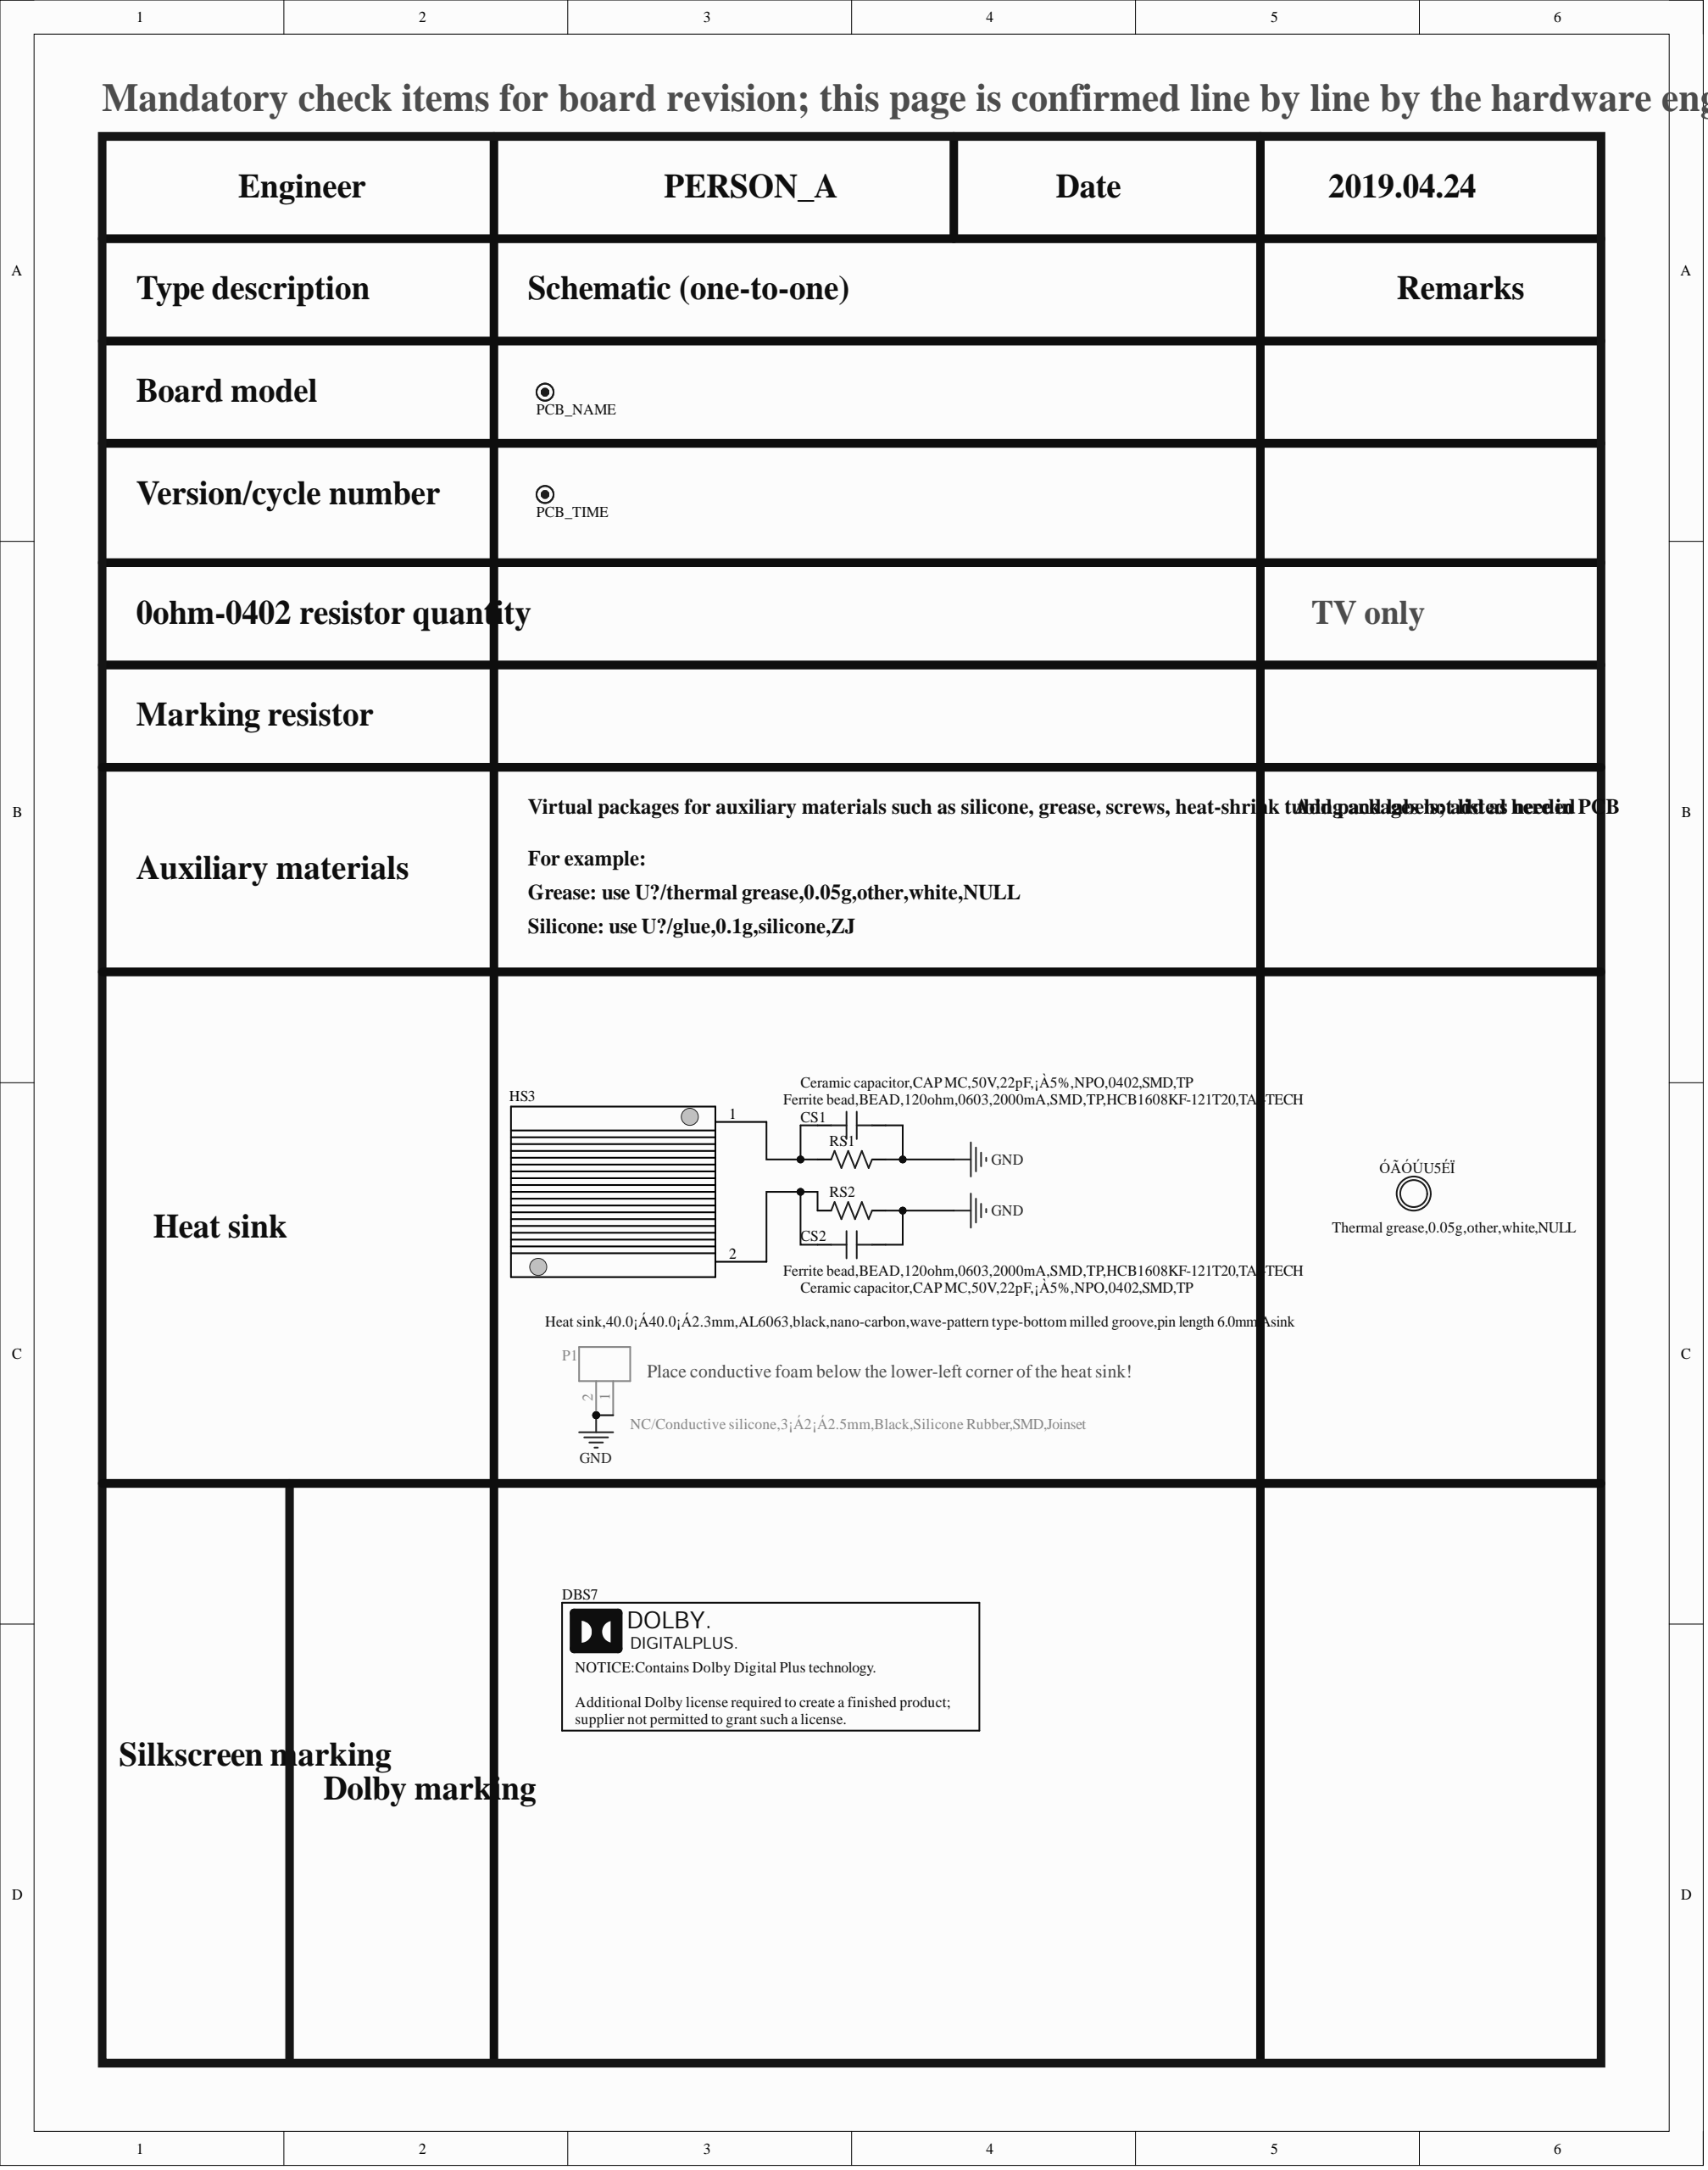Circuit board | Altium Designer | 951 parts | 509 nets | one sheet of the schematic
Parts on this sheet (reference | value | footprint):
CS1 | Ceramic capacitor,CAP MC,50V,22pF,¡À5%,NPO,0402,SMD,TP | C0402
CS2 | Ceramic capacitor,CAP MC,50V,22pF,¡À5%,NPO,0402,SMD,TP | C0402
DBS7 | DOLBY PLUS | DOLBY PLUS-SILK
HS3 | Heat sink,40.0¡Á40.0¡Á2.3mm,AL6063,black,nano-carbon,wave-pattern type-bottom milled groove,pin length 6.0mm,Asink | HS(40*40*2.3)-1
RS1 | Ferrite bead,BEAD,120ohm,0603,2000mA,SMD,TP,HCB1608KF-121T20,TAI-TECH | R0603
RS2 | Ferrite bead,BEAD,120ohm,0603,2000mA,SMD,TP,HCB1608KF-121T20,TAI-TECH | R0603
Nets of these parts (net: part-pin ...):
NetCS2_1: CS2-1 HS3-2 RS2-1
NetCS1_1: CS1-1 HS3-1 RS1-2
GND: CS1-2 CS2-2 RS1-1 RS2-2